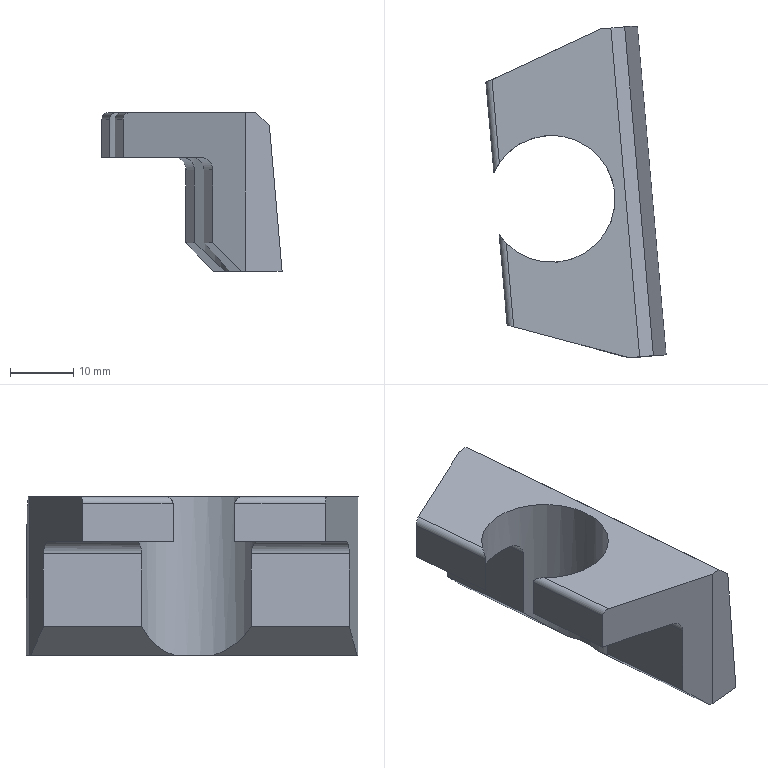Part | NX | features solid 2 | 1 solid | 21 faces | box 28.396 x 52.31 x 25 mm | volume 12914 mm3 | plane 16 | cylinder 5 | commonest cylinder face diameters 2 x2 4 x2 20 x1
STEP:
#1=CARTESIAN_POINT('',(-491.335,-14.427,136.998));
#2=VERTEX_POINT('',#1);
#3=CARTESIAN_POINT('',(-492.363,-14.151,135.998));
#4=VERTEX_POINT('',#3);
#5=CARTESIAN_POINT('',(-491.335,-14.427,135.998));
#6=DIRECTION('',(0.2588,0.9659,0.0000232));
#7=DIRECTION('',(0.9659,-0.2588,0.00006374));
#8=AXIS2_PLACEMENT_3D('',#5,#6,#7);
#9=ELLIPSE('',#8,1.064,1.);
#10=EDGE_CURVE('',#2,#4,#9,.F.);
#11=ORIENTED_EDGE('',*,*,#10,.F.);
#12=CARTESIAN_POINT('',(-492.485,-1.281,136.998));
#13=VERTEX_POINT('',#12);
#14=CARTESIAN_POINT('',(-495.305,30.949,136.998));
#15=DIRECTION('',(0.08716,-0.9962,0.));
#16=VECTOR('',#15,1000.);
#17=LINE('',#14,#16);
#18=EDGE_CURVE('',#13,#2,#17,.T.);
#19=ORIENTED_EDGE('',*,*,#18,.F.);
#20=CARTESIAN_POINT('',(-493.609,0.08901,135.998));
#21=VERTEX_POINT('',#20);
#22=CARTESIAN_POINT('',(-493.609,0.08901,135.998));
#23=CARTESIAN_POINT('',(-493.609,0.08901,136.185));
#24=CARTESIAN_POINT('',(-493.485,-0.0932,136.513));
#25=CARTESIAN_POINT('',(-493.102,-0.6057,136.883));
#26=CARTESIAN_POINT('',(-492.743,-1.017,136.998));
#27=CARTESIAN_POINT('',(-492.485,-1.281,136.998));
#28=B_SPLINE_CURVE_WITH_KNOTS('',3,(#22,#23,#24,#25,#26,#27),.UNSPECIFIED.,.F.,.F.,(4,1,1,4),(0.,0.0005521,0.001104,0.002208),.UNSPECIFIED.);
#29=EDGE_CURVE('',#21,#13,#28,.T.);
#30=ORIENTED_EDGE('',*,*,#29,.F.);
#31=CARTESIAN_POINT('',(-496.301,30.862,135.998));
#32=DIRECTION('',(0.08716,-0.9962,0.));
#33=VECTOR('',#32,1000.);
#34=LINE('',#31,#33);
#35=EDGE_CURVE('',#21,#4,#34,.T.);
#36=ORIENTED_EDGE('',*,*,#35,.T.);
#37=EDGE_LOOP('',(#11,#19,#30,#36));
#38=FACE_BOUND('',#37,.T.);
#39=CARTESIAN_POINT('',(-495.305,30.949,135.998));
#40=DIRECTION('',(0.08716,-0.9962,0.));
#41=DIRECTION('',(0.,0.,-1.));
#42=AXIS2_PLACEMENT_3D('',#39,#40,#41);
#43=CYLINDRICAL_SURFACE('',#42,1.);
#44=ADVANCED_FACE('',(#38),#43,.T.);
#45=CARTESIAN_POINT('',(-495.707,24.073,135.998));
#46=VERTEX_POINT('',#45);
#47=CARTESIAN_POINT('',(-494.461,9.833,135.998));
#48=VERTEX_POINT('',#47);
#49=CARTESIAN_POINT('',(-496.301,30.862,135.998));
#50=DIRECTION('',(0.08716,-0.9962,0.));
#51=VECTOR('',#50,1000.);
#52=LINE('',#49,#51);
#53=EDGE_CURVE('',#46,#48,#52,.T.);
#54=ORIENTED_EDGE('',*,*,#53,.F.);
#55=CARTESIAN_POINT('',(-495.707,24.073,129.998));
#56=VERTEX_POINT('',#55);
#57=CARTESIAN_POINT('',(-495.707,24.073,129.998));
#58=DIRECTION('',(0.,0.,-1.));
#59=VECTOR('',#58,1000.);
#60=LINE('',#57,#59);
#61=EDGE_CURVE('',#46,#56,#60,.T.);
#62=ORIENTED_EDGE('',*,*,#61,.T.);
#63=CARTESIAN_POINT('',(-494.461,9.833,129.998));
#64=VERTEX_POINT('',#63);
#65=CARTESIAN_POINT('',(-496.301,30.862,129.998));
#66=DIRECTION('',(0.08716,-0.9962,0.));
#67=VECTOR('',#66,1000.);
#68=LINE('',#65,#67);
#69=EDGE_CURVE('',#56,#64,#68,.T.);
#70=ORIENTED_EDGE('',*,*,#69,.T.);
#71=CARTESIAN_POINT('',(-494.461,9.833,87.));
#72=DIRECTION('',(0.,0.,1.));
#73=VECTOR('',#72,1000.);
#74=LINE('',#71,#73);
#75=EDGE_CURVE('',#64,#48,#74,.T.);
#76=ORIENTED_EDGE('',*,*,#75,.T.);
#77=EDGE_LOOP('',(#54,#62,#70,#76));
#78=FACE_BOUND('',#77,.T.);
#79=CARTESIAN_POINT('',(-496.301,30.862,129.998));
#80=DIRECTION('',(0.9962,0.08716,0.));
#81=DIRECTION('',(0.,0.,-1.));
#82=AXIS2_PLACEMENT_3D('',#79,#80,#81);
#83=PLANE('',#82);
#84=ADVANCED_FACE('',(#78),#83,.F.);
#85=CARTESIAN_POINT('',(-484.399,29.346,129.998));
#86=VERTEX_POINT('',#85);
#87=CARTESIAN_POINT('',(-493.595,25.058,129.998));
#88=DIRECTION('',(-0.9063,-0.4226,0.));
#89=VECTOR('',#88,1000.);
#90=LINE('',#87,#89);
#91=EDGE_CURVE('',#86,#56,#90,.T.);
#92=ORIENTED_EDGE('',*,*,#91,.F.);
#93=CARTESIAN_POINT('',(-483.187,15.485,129.998));
#94=VERTEX_POINT('',#93);
#95=CARTESIAN_POINT('',(-484.621,31.884,129.998));
#96=DIRECTION('',(0.08716,-0.9962,0.));
#97=VECTOR('',#96,1000.);
#98=LINE('',#95,#97);
#99=EDGE_CURVE('',#86,#94,#98,.T.);
#100=ORIENTED_EDGE('',*,*,#99,.T.);
#101=CARTESIAN_POINT('',(-485.346,5.721,129.998));
#102=DIRECTION('',(0.,0.,-1.));
#103=DIRECTION('',(-0.9962,-0.08716,0.));
#104=AXIS2_PLACEMENT_3D('',#101,#102,#103);
#105=CIRCLE('',#104,10.);
#106=EDGE_CURVE('',#64,#94,#105,.T.);
#107=ORIENTED_EDGE('',*,*,#106,.F.);
#108=ORIENTED_EDGE('',*,*,#69,.F.);
#109=EDGE_LOOP('',(#92,#100,#107,#108));
#110=FACE_BOUND('',#109,.T.);
#111=CARTESIAN_POINT('',(-496.301,30.862,129.998));
#112=DIRECTION('',(0.,0.,-1.));
#113=DIRECTION('',(-0.9962,-0.08716,0.));
#114=AXIS2_PLACEMENT_3D('',#111,#112,#113);
#115=PLANE('',#114);
#116=ADVANCED_FACE('',(#110),#115,.T.);
#117=CARTESIAN_POINT('',(-479.608,-2.469,127.998));
#118=VERTEX_POINT('',#117);
#119=CARTESIAN_POINT('',(-478.256,-17.931,127.998));
#120=VERTEX_POINT('',#119);
#121=CARTESIAN_POINT('',(-482.629,32.058,127.998));
#122=DIRECTION('',(0.08716,-0.9962,0.));
#123=VECTOR('',#122,1000.);
#124=LINE('',#121,#123);
#125=EDGE_CURVE('',#118,#120,#124,.T.);
#126=ORIENTED_EDGE('',*,*,#125,.T.);
#127=CARTESIAN_POINT('',(-480.311,-17.38,129.998));
#128=VERTEX_POINT('',#127);
#129=CARTESIAN_POINT('',(-480.311,-17.38,127.998));
#130=DIRECTION('',(0.2588,0.9659,0.0000232));
#131=DIRECTION('',(0.9659,-0.2588,0.00006374));
#132=AXIS2_PLACEMENT_3D('',#129,#130,#131);
#133=ELLIPSE('',#132,2.128,2.);
#134=EDGE_CURVE('',#120,#128,#133,.F.);
#135=ORIENTED_EDGE('',*,*,#134,.T.);
#136=CARTESIAN_POINT('',(-481.524,-3.52,129.998));
#137=VERTEX_POINT('',#136);
#138=CARTESIAN_POINT('',(-484.621,31.884,129.998));
#139=DIRECTION('',(0.08716,-0.9962,0.));
#140=VECTOR('',#139,1000.);
#141=LINE('',#138,#140);
#142=EDGE_CURVE('',#137,#128,#141,.T.);
#143=ORIENTED_EDGE('',*,*,#142,.F.);
#144=CARTESIAN_POINT('',(-481.524,-3.52,129.998));
#145=CARTESIAN_POINT('',(-480.504,-3.098,129.998));
#146=CARTESIAN_POINT('',(-479.608,-2.469,129.104));
#147=CARTESIAN_POINT('',(-479.608,-2.469,127.998));
#148=B_SPLINE_CURVE_WITH_KNOTS('',3,(#144,#145,#146,#147),.UNSPECIFIED.,.F.,.F.,(4,4),(0.,0.003262),.UNSPECIFIED.);
#149=EDGE_CURVE('',#137,#118,#148,.T.);
#150=ORIENTED_EDGE('',*,*,#149,.T.);
#151=EDGE_LOOP('',(#126,#135,#143,#150));
#152=FACE_BOUND('',#151,.T.);
#153=CARTESIAN_POINT('',(-484.621,31.884,127.998));
#154=DIRECTION('',(0.08716,-0.9962,0.));
#155=DIRECTION('',(0.,0.,-1.));
#156=AXIS2_PLACEMENT_3D('',#153,#154,#155);
#157=CYLINDRICAL_SURFACE('',#156,2.);
#158=ADVANCED_FACE('',(#152),#157,.F.);
#159=CARTESIAN_POINT('',(-482.471,30.246,127.998));
#160=VERTEX_POINT('',#159);
#161=CARTESIAN_POINT('',(-481.118,14.783,127.998));
#162=VERTEX_POINT('',#161);
#163=CARTESIAN_POINT('',(-482.629,32.058,127.998));
#164=DIRECTION('',(0.08716,-0.9962,0.));
#165=VECTOR('',#164,1000.);
#166=LINE('',#163,#165);
#167=EDGE_CURVE('',#160,#162,#166,.T.);
#168=ORIENTED_EDGE('',*,*,#167,.F.);
#169=CARTESIAN_POINT('',(-482.471,30.246,116.498));
#170=VERTEX_POINT('',#169);
#171=CARTESIAN_POINT('',(-482.471,30.246,116.498));
#172=DIRECTION('',(0.,0.,-1.));
#173=VECTOR('',#172,1000.);
#174=LINE('',#171,#173);
#175=EDGE_CURVE('',#160,#170,#174,.T.);
#176=ORIENTED_EDGE('',*,*,#175,.T.);
#177=CARTESIAN_POINT('',(-481.118,14.783,116.498));
#178=VERTEX_POINT('',#177);
#179=CARTESIAN_POINT('',(-482.629,32.058,116.498));
#180=DIRECTION('',(0.08716,-0.9962,0.));
#181=VECTOR('',#180,1000.);
#182=LINE('',#179,#181);
#183=EDGE_CURVE('',#170,#178,#182,.T.);
#184=ORIENTED_EDGE('',*,*,#183,.T.);
#185=CARTESIAN_POINT('',(-481.118,14.783,87.));
#186=DIRECTION('',(0.,0.,1.));
#187=VECTOR('',#186,1000.);
#188=LINE('',#185,#187);
#189=EDGE_CURVE('',#178,#162,#188,.T.);
#190=ORIENTED_EDGE('',*,*,#189,.T.);
#191=EDGE_LOOP('',(#168,#176,#184,#190));
#192=FACE_BOUND('',#191,.T.);
#193=CARTESIAN_POINT('',(-482.629,32.058,116.498));
#194=DIRECTION('',(0.9962,0.08716,0.));
#195=DIRECTION('',(0.,0.,-1.));
#196=AXIS2_PLACEMENT_3D('',#193,#194,#195);
#197=PLANE('',#196);
#198=ADVANCED_FACE('',(#192),#197,.F.);
#199=CARTESIAN_POINT('',(-478.13,32.27,111.998));
#200=VERTEX_POINT('',#199);
#201=CARTESIAN_POINT('',(-482.171,30.385,116.187));
#202=DIRECTION('',(-0.6605,-0.308,0.6848));
#203=VECTOR('',#202,1000.);
#204=LINE('',#201,#203);
#205=EDGE_CURVE('',#200,#170,#204,.T.);
#206=ORIENTED_EDGE('',*,*,#205,.F.);
#207=CARTESIAN_POINT('',(-476.152,9.655,111.998));
#208=VERTEX_POINT('',#207);
#209=CARTESIAN_POINT('',(-478.146,32.45,111.998));
#210=DIRECTION('',(0.08716,-0.9962,0.));
#211=VECTOR('',#210,1000.);
#212=LINE('',#209,#211);
#213=EDGE_CURVE('',#200,#208,#212,.T.);
#214=ORIENTED_EDGE('',*,*,#213,.T.);
#215=CARTESIAN_POINT('',(-485.346,5.721,121.499));
#216=DIRECTION('',(-0.7044,-0.06163,-0.7071));
#217=DIRECTION('',(-0.7044,-0.06163,0.7071));
#218=AXIS2_PLACEMENT_3D('',#215,#216,#217);
#219=ELLIPSE('',#218,14.142,10.);
#220=EDGE_CURVE('',#178,#208,#219,.T.);
#221=ORIENTED_EDGE('',*,*,#220,.F.);
#222=ORIENTED_EDGE('',*,*,#183,.F.);
#223=EDGE_LOOP('',(#206,#214,#221,#222));
#224=FACE_BOUND('',#223,.T.);
#225=CARTESIAN_POINT('',(-482.629,32.058,116.498));
#226=DIRECTION('',(-0.7044,-0.06163,-0.7071));
#227=DIRECTION('',(-0.7044,-0.06163,0.7071));
#228=AXIS2_PLACEMENT_3D('',#225,#226,#227);
#229=PLANE('',#228);
#230=ADVANCED_FACE('',(#224),#229,.T.);
#231=CARTESIAN_POINT('',(-494.743,24.523,136.998));
#232=VERTEX_POINT('',#231);
#233=CARTESIAN_POINT('',(-494.743,24.523,135.998));
#234=DIRECTION('',(0.4226,-0.9063,0.));
#235=DIRECTION('',(-0.9063,-0.4226,0.));
#236=AXIS2_PLACEMENT_3D('',#233,#234,#235);
#237=ELLIPSE('',#236,1.064,1.);
#238=EDGE_CURVE('',#46,#232,#237,.F.);
#239=ORIENTED_EDGE('',*,*,#238,.F.);
#240=ORIENTED_EDGE('',*,*,#53,.T.);
#241=CARTESIAN_POINT('',(-493.592,11.377,136.998));
#242=VERTEX_POINT('',#241);
#243=CARTESIAN_POINT('',(-493.592,11.377,136.998));
#244=CARTESIAN_POINT('',(-493.801,11.073,136.998));
#245=CARTESIAN_POINT('',(-494.164,10.481,136.861));
#246=CARTESIAN_POINT('',(-494.461,9.833,136.371));
#247=CARTESIAN_POINT('',(-494.461,9.833,135.998));
#248=B_SPLINE_CURVE_WITH_KNOTS('',3,(#243,#244,#245,#246,#247),.UNSPECIFIED.,.F.,.F.,(4,1,4),(0.,0.001092,0.002183),.UNSPECIFIED.);
#249=EDGE_CURVE('',#242,#48,#248,.T.);
#250=ORIENTED_EDGE('',*,*,#249,.F.);
#251=CARTESIAN_POINT('',(-495.305,30.949,136.998));
#252=DIRECTION('',(0.08716,-0.9962,0.));
#253=VECTOR('',#252,1000.);
#254=LINE('',#251,#253);
#255=EDGE_CURVE('',#232,#242,#254,.T.);
#256=ORIENTED_EDGE('',*,*,#255,.F.);
#257=EDGE_LOOP('',(#239,#240,#250,#256));
#258=FACE_BOUND('',#257,.T.);
#259=CARTESIAN_POINT('',(-495.305,30.949,135.998));
#260=DIRECTION('',(0.08716,-0.9962,0.));
#261=DIRECTION('',(0.,0.,-1.));
#262=AXIS2_PLACEMENT_3D('',#259,#260,#261);
#263=CYLINDRICAL_SURFACE('',#262,1.);
#264=ADVANCED_FACE('',(#258),#263,.T.);
#265=CARTESIAN_POINT('',(-493.609,0.08901,129.998));
#266=VERTEX_POINT('',#265);
#267=CARTESIAN_POINT('',(-492.363,-14.151,129.998));
#268=VERTEX_POINT('',#267);
#269=CARTESIAN_POINT('',(-496.301,30.862,129.998));
#270=DIRECTION('',(0.08716,-0.9962,0.));
#271=VECTOR('',#270,1000.);
#272=LINE('',#269,#271);
#273=EDGE_CURVE('',#266,#268,#272,.T.);
#274=ORIENTED_EDGE('',*,*,#273,.T.);
#275=CARTESIAN_POINT('',(-492.363,-14.151,129.997));
#276=DIRECTION('',(0.000002152,-0.00002459,1.));
#277=VECTOR('',#276,1000.);
#278=LINE('',#275,#277);
#279=EDGE_CURVE('',#268,#4,#278,.T.);
#280=ORIENTED_EDGE('',*,*,#279,.T.);
#281=ORIENTED_EDGE('',*,*,#35,.F.);
#282=CARTESIAN_POINT('',(-493.609,0.08901,87.));
#283=DIRECTION('',(0.,0.,1.));
#284=VECTOR('',#283,1000.);
#285=LINE('',#282,#284);
#286=EDGE_CURVE('',#21,#266,#285,.F.);
#287=ORIENTED_EDGE('',*,*,#286,.T.);
#288=EDGE_LOOP('',(#274,#280,#281,#287));
#289=FACE_BOUND('',#288,.T.);
#290=CARTESIAN_POINT('',(-496.301,30.862,129.998));
#291=DIRECTION('',(0.9962,0.08716,0.));
#292=DIRECTION('',(0.,0.,-1.));
#293=AXIS2_PLACEMENT_3D('',#290,#291,#292);
#294=PLANE('',#293);
#295=ADVANCED_FACE('',(#289),#294,.F.);
#296=CARTESIAN_POINT('',(-507.29,-10.151,129.998));
#297=DIRECTION('',(0.9659,-0.2588,0.));
#298=VECTOR('',#297,1000.);
#299=LINE('',#296,#298);
#300=EDGE_CURVE('',#268,#128,#299,.T.);
#301=ORIENTED_EDGE('',*,*,#300,.F.);
#302=ORIENTED_EDGE('',*,*,#273,.F.);
#303=CARTESIAN_POINT('',(-485.346,5.721,129.998));
#304=DIRECTION('',(0.,0.,-1.));
#305=DIRECTION('',(-0.9962,-0.08716,0.));
#306=AXIS2_PLACEMENT_3D('',#303,#304,#305);
#307=CIRCLE('',#306,10.);
#308=EDGE_CURVE('',#137,#266,#307,.T.);
#309=ORIENTED_EDGE('',*,*,#308,.F.);
#310=ORIENTED_EDGE('',*,*,#142,.T.);
#311=EDGE_LOOP('',(#301,#302,#309,#310));
#312=FACE_BOUND('',#311,.T.);
#313=CARTESIAN_POINT('',(-496.301,30.862,129.998));
#314=DIRECTION('',(0.,0.,-1.));
#315=DIRECTION('',(-0.9962,-0.08716,0.));
#316=AXIS2_PLACEMENT_3D('',#313,#314,#315);
#317=PLANE('',#316);
#318=ADVANCED_FACE('',(#312),#317,.T.);
#319=ORIENTED_EDGE('',*,*,#99,.F.);
#320=CARTESIAN_POINT('',(-484.399,29.346,127.998));
#321=DIRECTION('',(0.4226,-0.9063,0.));
#322=DIRECTION('',(-0.9063,-0.4226,0.));
#323=AXIS2_PLACEMENT_3D('',#320,#321,#322);
#324=ELLIPSE('',#323,2.128,2.);
#325=EDGE_CURVE('',#86,#160,#324,.F.);
#326=ORIENTED_EDGE('',*,*,#325,.T.);
#327=ORIENTED_EDGE('',*,*,#167,.T.);
#328=CARTESIAN_POINT('',(-481.118,14.783,127.998));
#329=CARTESIAN_POINT('',(-481.118,14.783,129.102));
#330=CARTESIAN_POINT('',(-482.111,15.247,129.998));
#331=CARTESIAN_POINT('',(-483.187,15.485,129.998));
#332=B_SPLINE_CURVE_WITH_KNOTS('',3,(#328,#329,#330,#331),.UNSPECIFIED.,.F.,.F.,(4,4),(0.,0.003262),.UNSPECIFIED.);
#333=EDGE_CURVE('',#162,#94,#332,.T.);
#334=ORIENTED_EDGE('',*,*,#333,.T.);
#335=EDGE_LOOP('',(#319,#326,#327,#334));
#336=FACE_BOUND('',#335,.T.);
#337=CARTESIAN_POINT('',(-484.621,31.884,127.998));
#338=DIRECTION('',(0.08716,-0.9962,0.));
#339=DIRECTION('',(0.,0.,-1.));
#340=AXIS2_PLACEMENT_3D('',#337,#338,#339);
#341=CYLINDRICAL_SURFACE('',#340,2.);
#342=ADVANCED_FACE('',(#336),#341,.F.);
#343=CARTESIAN_POINT('',(-479.608,-2.469,116.498));
#344=VERTEX_POINT('',#343);
#345=CARTESIAN_POINT('',(-478.256,-17.931,116.498));
#346=VERTEX_POINT('',#345);
#347=CARTESIAN_POINT('',(-482.629,32.058,116.498));
#348=DIRECTION('',(0.08716,-0.9962,0.));
#349=VECTOR('',#348,1000.);
#350=LINE('',#347,#349);
#351=EDGE_CURVE('',#344,#346,#350,.T.);
#352=ORIENTED_EDGE('',*,*,#351,.T.);
#353=CARTESIAN_POINT('',(-478.256,-17.931,116.497));
#354=DIRECTION('',(0.000002152,-0.00002459,1.));
#355=VECTOR('',#354,1000.);
#356=LINE('',#353,#355);
#357=EDGE_CURVE('',#346,#120,#356,.T.);
#358=ORIENTED_EDGE('',*,*,#357,.T.);
#359=ORIENTED_EDGE('',*,*,#125,.F.);
#360=CARTESIAN_POINT('',(-479.608,-2.469,87.));
#361=DIRECTION('',(0.,0.,1.));
#362=VECTOR('',#361,1000.);
#363=LINE('',#360,#362);
#364=EDGE_CURVE('',#118,#344,#363,.F.);
#365=ORIENTED_EDGE('',*,*,#364,.T.);
#366=EDGE_LOOP('',(#352,#358,#359,#365));
#367=FACE_BOUND('',#366,.T.);
#368=CARTESIAN_POINT('',(-482.629,32.058,116.498));
#369=DIRECTION('',(0.9962,0.08716,0.));
#370=DIRECTION('',(0.,0.,-1.));
#371=AXIS2_PLACEMENT_3D('',#368,#369,#370);
#372=PLANE('',#371);
#373=ADVANCED_FACE('',(#367),#372,.F.);
#374=CARTESIAN_POINT('',(-473.63,-19.17,111.998));
#375=VERTEX_POINT('',#374);
#376=CARTESIAN_POINT('',(-487.059,-15.572,125.062));
#377=DIRECTION('',(0.7039,-0.1886,-0.6848));
#378=VECTOR('',#377,1000.);
#379=LINE('',#376,#378);
#380=EDGE_CURVE('',#346,#375,#379,.T.);
#381=ORIENTED_EDGE('',*,*,#380,.F.);
#382=ORIENTED_EDGE('',*,*,#351,.F.);
#383=CARTESIAN_POINT('',(-475.608,3.443,111.998));
#384=VERTEX_POINT('',#383);
#385=CARTESIAN_POINT('',(-485.346,5.721,121.499));
#386=DIRECTION('',(-0.7044,-0.06163,-0.7071));
#387=DIRECTION('',(-0.7044,-0.06163,0.7071));
#388=AXIS2_PLACEMENT_3D('',#385,#386,#387);
#389=ELLIPSE('',#388,14.142,10.);
#390=EDGE_CURVE('',#384,#344,#389,.T.);
#391=ORIENTED_EDGE('',*,*,#390,.F.);
#392=CARTESIAN_POINT('',(-478.146,32.45,111.998));
#393=DIRECTION('',(0.08716,-0.9962,0.));
#394=VECTOR('',#393,1000.);
#395=LINE('',#392,#394);
#396=EDGE_CURVE('',#384,#375,#395,.T.);
#397=ORIENTED_EDGE('',*,*,#396,.T.);
#398=EDGE_LOOP('',(#381,#382,#391,#397));
#399=FACE_BOUND('',#398,.T.);
#400=CARTESIAN_POINT('',(-482.629,32.058,116.498));
#401=DIRECTION('',(-0.7044,-0.06163,-0.7071));
#402=DIRECTION('',(-0.7044,-0.06163,0.7071));
#403=AXIS2_PLACEMENT_3D('',#400,#401,#402);
#404=PLANE('',#403);
#405=ADVANCED_FACE('',(#399),#404,.T.);
#406=CARTESIAN_POINT('',(-477.65,32.494,111.998));
#407=VERTEX_POINT('',#406);
#408=CARTESIAN_POINT('',(-478.074,32.296,111.998));
#409=DIRECTION('',(-0.9063,-0.4226,0.));
#410=VECTOR('',#409,1000.);
#411=LINE('',#408,#410);
#412=EDGE_CURVE('',#407,#200,#411,.T.);
#413=ORIENTED_EDGE('',*,*,#412,.F.);
#414=CARTESIAN_POINT('',(-471.843,33.002,111.998));
#415=VERTEX_POINT('',#414);
#416=CARTESIAN_POINT('',(-478.146,32.45,111.998));
#417=DIRECTION('',(0.9962,0.08716,0.));
#418=VECTOR('',#417,1000.);
#419=LINE('',#416,#418);
#420=EDGE_CURVE('',#407,#415,#419,.T.);
#421=ORIENTED_EDGE('',*,*,#420,.T.);
#422=CARTESIAN_POINT('',(-467.311,-18.8,111.998));
#423=VERTEX_POINT('',#422);
#424=CARTESIAN_POINT('',(-471.843,33.002,111.998));
#425=DIRECTION('',(0.08716,-0.9962,0.));
#426=VECTOR('',#425,1000.);
#427=LINE('',#424,#426);
#428=EDGE_CURVE('',#415,#423,#427,.T.);
#429=ORIENTED_EDGE('',*,*,#428,.T.);
#430=CARTESIAN_POINT('',(-473.114,-19.308,111.998));
#431=VERTEX_POINT('',#430);
#432=CARTESIAN_POINT('',(-473.614,-19.352,111.998));
#433=DIRECTION('',(0.9962,0.08716,0.));
#434=VECTOR('',#433,1000.);
#435=LINE('',#432,#434);
#436=EDGE_CURVE('',#431,#423,#435,.T.);
#437=ORIENTED_EDGE('',*,*,#436,.F.);
#438=CARTESIAN_POINT('',(-490.749,-14.583,111.998));
#439=DIRECTION('',(0.9659,-0.2588,0.));
#440=VECTOR('',#439,1000.);
#441=LINE('',#438,#440);
#442=EDGE_CURVE('',#375,#431,#441,.T.);
#443=ORIENTED_EDGE('',*,*,#442,.F.);
#444=ORIENTED_EDGE('',*,*,#396,.F.);
#445=CARTESIAN_POINT('',(-485.346,5.721,111.998));
#446=DIRECTION('',(0.,0.,-1.));
#447=DIRECTION('',(-0.9962,-0.08716,0.));
#448=AXIS2_PLACEMENT_3D('',#445,#446,#447);
#449=CIRCLE('',#448,10.);
#450=EDGE_CURVE('',#208,#384,#449,.T.);
#451=ORIENTED_EDGE('',*,*,#450,.F.);
#452=ORIENTED_EDGE('',*,*,#213,.F.);
#453=EDGE_LOOP('',(#413,#421,#429,#437,#443,#444,#451,#452));
#454=FACE_BOUND('',#453,.T.);
#455=CARTESIAN_POINT('',(-478.146,32.45,111.998));
#456=DIRECTION('',(0.,0.,-1.));
#457=DIRECTION('',(-0.9962,-0.08716,0.));
#458=AXIS2_PLACEMENT_3D('',#455,#456,#457);
#459=PLANE('',#458);
#460=ADVANCED_FACE('',(#454),#459,.T.);
#461=CARTESIAN_POINT('',(-469.316,-18.976,135.006));
#462=VERTEX_POINT('',#461);
#463=CARTESIAN_POINT('',(-469.316,-18.976,135.006));
#464=DIRECTION('',(0.08682,0.007596,-0.9962));
#465=VECTOR('',#464,1000.);
#466=LINE('',#463,#465);
#467=EDGE_CURVE('',#462,#423,#466,.T.);
#468=ORIENTED_EDGE('',*,*,#467,.T.);
#469=ORIENTED_EDGE('',*,*,#428,.F.);
#470=CARTESIAN_POINT('',(-473.848,32.826,135.006));
#471=VERTEX_POINT('',#470);
#472=CARTESIAN_POINT('',(-473.848,32.826,135.006));
#473=DIRECTION('',(0.08682,0.007596,-0.9962));
#474=VECTOR('',#473,1000.);
#475=LINE('',#472,#474);
#476=EDGE_CURVE('',#471,#415,#475,.T.);
#477=ORIENTED_EDGE('',*,*,#476,.F.);
#478=CARTESIAN_POINT('',(-473.848,32.826,135.006));
#479=DIRECTION('',(0.08716,-0.9962,0.));
#480=VECTOR('',#479,1000.);
#481=LINE('',#478,#480);
#482=EDGE_CURVE('',#471,#462,#481,.T.);
#483=ORIENTED_EDGE('',*,*,#482,.T.);
#484=EDGE_LOOP('',(#468,#469,#477,#483));
#485=FACE_BOUND('',#484,.T.);
#486=CARTESIAN_POINT('',(-473.848,32.826,135.006));
#487=DIRECTION('',(-0.9924,-0.08682,-0.08716));
#488=DIRECTION('',(-0.08682,-0.007596,0.9962));
#489=AXIS2_PLACEMENT_3D('',#486,#487,#488);
#490=PLANE('',#489);
#491=ADVANCED_FACE('',(#485),#490,.F.);
#492=CARTESIAN_POINT('',(-471.482,-19.165,136.998));
#493=VERTEX_POINT('',#492);
#494=CARTESIAN_POINT('',(-471.482,-19.165,136.998));
#495=DIRECTION('',(0.7345,0.06426,-0.6756));
#496=VECTOR('',#495,1000.);
#497=LINE('',#494,#496);
#498=EDGE_CURVE('',#493,#462,#497,.T.);
#499=ORIENTED_EDGE('',*,*,#498,.T.);
#500=ORIENTED_EDGE('',*,*,#482,.F.);
#501=CARTESIAN_POINT('',(-476.014,32.637,136.998));
#502=VERTEX_POINT('',#501);
#503=CARTESIAN_POINT('',(-476.014,32.637,136.998));
#504=DIRECTION('',(0.7345,0.06426,-0.6756));
#505=VECTOR('',#504,1000.);
#506=LINE('',#503,#505);
#507=EDGE_CURVE('',#502,#471,#506,.T.);
#508=ORIENTED_EDGE('',*,*,#507,.F.);
#509=CARTESIAN_POINT('',(-476.014,32.637,136.998));
#510=DIRECTION('',(0.08716,-0.9962,0.));
#511=VECTOR('',#510,1000.);
#512=LINE('',#509,#511);
#513=EDGE_CURVE('',#502,#493,#512,.T.);
#514=ORIENTED_EDGE('',*,*,#513,.T.);
#515=EDGE_LOOP('',(#499,#500,#508,#514));
#516=FACE_BOUND('',#515,.T.);
#517=CARTESIAN_POINT('',(-476.014,32.637,136.998));
#518=DIRECTION('',(-0.673,-0.05888,-0.7373));
#519=DIRECTION('',(-0.7345,-0.06426,0.6756));
#520=AXIS2_PLACEMENT_3D('',#517,#518,#519);
#521=PLANE('',#520);
#522=ADVANCED_FACE('',(#516),#521,.F.);
#523=CARTESIAN_POINT('',(-477.65,32.494,136.998));
#524=VERTEX_POINT('',#523);
#525=CARTESIAN_POINT('',(-495.305,30.949,136.998));
#526=DIRECTION('',(0.9962,0.08716,0.));
#527=VECTOR('',#526,1000.);
#528=LINE('',#525,#527);
#529=EDGE_CURVE('',#524,#502,#528,.T.);
#530=ORIENTED_EDGE('',*,*,#529,.F.);
#531=CARTESIAN_POINT('',(-492.743,25.456,136.998));
#532=DIRECTION('',(-0.9063,-0.4226,0.));
#533=VECTOR('',#532,1000.);
#534=LINE('',#531,#533);
#535=EDGE_CURVE('',#524,#232,#534,.T.);
#536=ORIENTED_EDGE('',*,*,#535,.T.);
#537=ORIENTED_EDGE('',*,*,#255,.T.);
#538=CARTESIAN_POINT('',(-485.346,5.721,136.998));
#539=DIRECTION('',(0.,0.,-1.));
#540=DIRECTION('',(-0.9962,-0.08716,0.));
#541=AXIS2_PLACEMENT_3D('',#538,#539,#540);
#542=CIRCLE('',#541,10.);
#543=EDGE_CURVE('',#242,#13,#542,.T.);
#544=ORIENTED_EDGE('',*,*,#543,.T.);
#545=ORIENTED_EDGE('',*,*,#18,.T.);
#546=CARTESIAN_POINT('',(-473.116,-19.308,136.998));
#547=VERTEX_POINT('',#546);
#548=CARTESIAN_POINT('',(-506.383,-10.394,136.998));
#549=DIRECTION('',(0.9659,-0.2588,0.));
#550=VECTOR('',#549,1000.);
#551=LINE('',#548,#550);
#552=EDGE_CURVE('',#2,#547,#551,.T.);
#553=ORIENTED_EDGE('',*,*,#552,.T.);
#554=CARTESIAN_POINT('',(-490.773,-20.853,136.998));
#555=DIRECTION('',(0.9962,0.08716,0.));
#556=VECTOR('',#555,1000.);
#557=LINE('',#554,#556);
#558=EDGE_CURVE('',#547,#493,#557,.T.);
#559=ORIENTED_EDGE('',*,*,#558,.T.);
#560=ORIENTED_EDGE('',*,*,#513,.F.);
#561=EDGE_LOOP('',(#530,#536,#537,#544,#545,#553,#559,#560));
#562=FACE_BOUND('',#561,.T.);
#563=CARTESIAN_POINT('',(-495.305,30.949,136.998));
#564=DIRECTION('',(0.,0.,-1.));
#565=DIRECTION('',(-0.9962,-0.08716,0.));
#566=AXIS2_PLACEMENT_3D('',#563,#564,#565);
#567=PLANE('',#566);
#568=ADVANCED_FACE('',(#562),#567,.F.);
#569=ORIENTED_EDGE('',*,*,#420,.F.);
#570=CARTESIAN_POINT('',(-477.65,32.494,135.998));
#571=DIRECTION('',(0.,0.,1.));
#572=VECTOR('',#571,1000.);
#573=LINE('',#570,#572);
#574=EDGE_CURVE('',#407,#524,#573,.T.);
#575=ORIENTED_EDGE('',*,*,#574,.T.);
#576=ORIENTED_EDGE('',*,*,#529,.T.);
#577=ORIENTED_EDGE('',*,*,#507,.T.);
#578=ORIENTED_EDGE('',*,*,#476,.T.);
#579=EDGE_LOOP('',(#569,#575,#576,#577,#578));
#580=FACE_BOUND('',#579,.T.);
#581=CARTESIAN_POINT('',(-495.305,30.949,135.998));
#582=DIRECTION('',(0.08716,-0.9962,0.));
#583=DIRECTION('',(0.,0.,-1.));
#584=AXIS2_PLACEMENT_3D('',#581,#582,#583);
#585=PLANE('',#584);
#586=ADVANCED_FACE('',(#580),#585,.F.);
#587=CARTESIAN_POINT('',(-473.116,-19.308,135.999));
#588=DIRECTION('',(-0.00006757,-0.000005911,1.));
#589=VECTOR('',#588,1000.);
#590=LINE('',#587,#589);
#591=EDGE_CURVE('',#431,#547,#590,.T.);
#592=ORIENTED_EDGE('',*,*,#591,.F.);
#593=ORIENTED_EDGE('',*,*,#436,.T.);
#594=ORIENTED_EDGE('',*,*,#467,.F.);
#595=ORIENTED_EDGE('',*,*,#498,.F.);
#596=ORIENTED_EDGE('',*,*,#558,.F.);
#597=EDGE_LOOP('',(#592,#593,#594,#595,#596));
#598=FACE_BOUND('',#597,.T.);
#599=CARTESIAN_POINT('',(-490.773,-20.853,135.998));
#600=DIRECTION('',(0.08716,-0.9962,0.));
#601=DIRECTION('',(0.,0.,-1.));
#602=AXIS2_PLACEMENT_3D('',#599,#600,#601);
#603=PLANE('',#602);
#604=ADVANCED_FACE('',(#598),#603,.T.);
#605=ORIENTED_EDGE('',*,*,#450,.T.);
#606=ORIENTED_EDGE('',*,*,#390,.T.);
#607=ORIENTED_EDGE('',*,*,#364,.F.);
#608=ORIENTED_EDGE('',*,*,#149,.F.);
#609=ORIENTED_EDGE('',*,*,#308,.T.);
#610=ORIENTED_EDGE('',*,*,#286,.F.);
#611=ORIENTED_EDGE('',*,*,#29,.T.);
#612=ORIENTED_EDGE('',*,*,#543,.F.);
#613=ORIENTED_EDGE('',*,*,#249,.T.);
#614=ORIENTED_EDGE('',*,*,#75,.F.);
#615=ORIENTED_EDGE('',*,*,#106,.T.);
#616=ORIENTED_EDGE('',*,*,#333,.F.);
#617=ORIENTED_EDGE('',*,*,#189,.F.);
#618=ORIENTED_EDGE('',*,*,#220,.T.);
#619=EDGE_LOOP('',(#605,#606,#607,#608,#609,#610,#611,#612,#613,#614,#615,#616,#617,#618));
#620=FACE_BOUND('',#619,.T.);
#621=CARTESIAN_POINT('',(-485.346,5.721,87.));
#622=DIRECTION('',(0.,0.,1.));
#623=DIRECTION('',(0.9962,0.08716,0.));
#624=AXIS2_PLACEMENT_3D('',#621,#622,#623);
#625=CYLINDRICAL_SURFACE('',#624,10.);
#626=ADVANCED_FACE('',(#620),#625,.F.);
#627=ORIENTED_EDGE('',*,*,#279,.F.);
#628=ORIENTED_EDGE('',*,*,#300,.T.);
#629=ORIENTED_EDGE('',*,*,#134,.F.);
#630=ORIENTED_EDGE('',*,*,#357,.F.);
#631=ORIENTED_EDGE('',*,*,#380,.T.);
#632=ORIENTED_EDGE('',*,*,#442,.T.);
#633=ORIENTED_EDGE('',*,*,#591,.T.);
#634=ORIENTED_EDGE('',*,*,#552,.F.);
#635=ORIENTED_EDGE('',*,*,#10,.T.);
#636=EDGE_LOOP('',(#627,#628,#629,#630,#631,#632,#633,#634,#635));
#637=FACE_BOUND('',#636,.T.);
#638=CARTESIAN_POINT('',(-498.815,-12.423,159.));
#639=DIRECTION('',(0.2588,0.9659,0.0000232));
#640=DIRECTION('',(-0.9659,0.2588,0.));
#641=AXIS2_PLACEMENT_3D('',#638,#639,#640);
#642=PLANE('',#641);
#643=ADVANCED_FACE('',(#637),#642,.F.);
#644=ORIENTED_EDGE('',*,*,#325,.F.);
#645=ORIENTED_EDGE('',*,*,#91,.T.);
#646=ORIENTED_EDGE('',*,*,#61,.F.);
#647=ORIENTED_EDGE('',*,*,#238,.T.);
#648=ORIENTED_EDGE('',*,*,#535,.F.);
#649=ORIENTED_EDGE('',*,*,#574,.F.);
#650=ORIENTED_EDGE('',*,*,#412,.T.);
#651=ORIENTED_EDGE('',*,*,#205,.T.);
#652=ORIENTED_EDGE('',*,*,#175,.F.);
#653=EDGE_LOOP('',(#644,#645,#646,#647,#648,#649,#650,#651,#652));
#654=FACE_BOUND('',#653,.T.);
#655=CARTESIAN_POINT('',(-501.761,21.25,159.));
#656=DIRECTION('',(0.4226,-0.9063,0.));
#657=DIRECTION('',(0.9063,0.4226,0.));
#658=AXIS2_PLACEMENT_3D('',#655,#656,#657);
#659=PLANE('',#658);
#660=ADVANCED_FACE('',(#654),#659,.F.);
#661=CLOSED_SHELL('',(#44,#84,#116,#158,#198,#230,#264,#295,#318,#342,#373,#405,#460,#491,#522,#568,#586,#604,#626,#643,#660));
#662=MANIFOLD_SOLID_BREP('',#661);
#663=(LENGTH_UNIT()NAMED_UNIT(*)SI_UNIT(.MILLI.,.METRE.));
#664=UNCERTAINTY_MEASURE_WITH_UNIT(LENGTH_MEASURE(0.0508),#663,'','');
#665=(NAMED_UNIT(*)PLANE_ANGLE_UNIT()SI_UNIT($,.RADIAN.));
#666=(NAMED_UNIT(*)SI_UNIT($,.STERADIAN.)SOLID_ANGLE_UNIT());
#667=(GEOMETRIC_REPRESENTATION_CONTEXT(3)GLOBAL_UNCERTAINTY_ASSIGNED_CONTEXT((#664))GLOBAL_UNIT_ASSIGNED_CONTEXT((#663,#665,#666))REPRESENTATION_CONTEXT('',''));
#668=ADVANCED_BREP_SHAPE_REPRESENTATION('',(#662),#667);